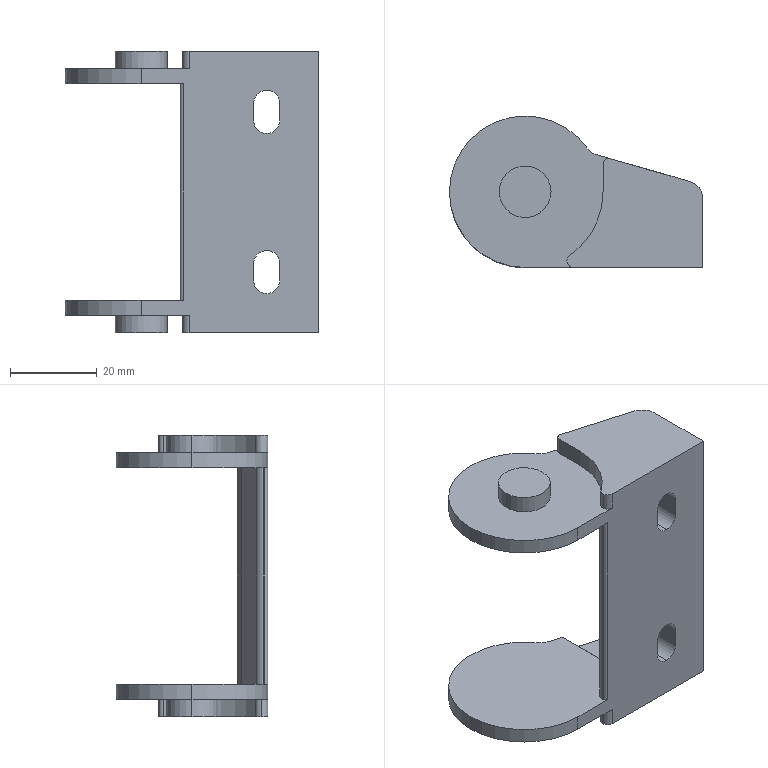Part | SolidWorks | features BaseBody 1 | 1 solid | 53 faces | box 58.5 x 35 x 65 mm | volume 23683 mm3 | cylinder 28 | plane 25 | commonest cylinder face diameters 6 x6 8 x4 11.95 x4 35 x4 3 x3 2.4 x2